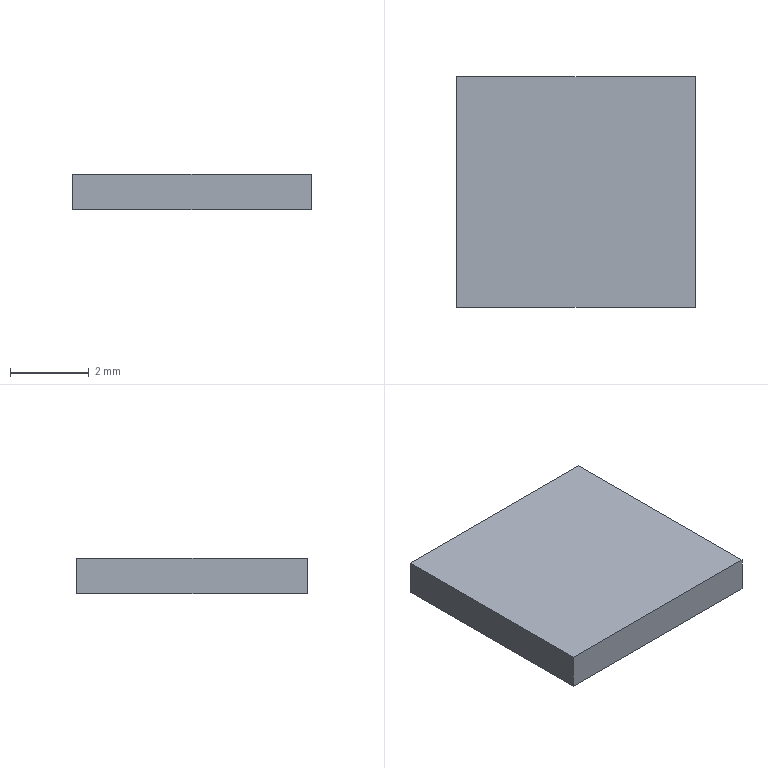Part | Creo | 1 solid | 6 faces | box 6.05 x 5.85 x 0.9 mm | volume 31.853 mm3 | plane 6
STEP:
#1=CARTESIAN_POINT('',(0.,0.,0.));
#2=DIRECTION('',(0.,0.,1.));
#3=DIRECTION('',(1.,0.,0.));
#4=AXIS2_PLACEMENT_3D('',#1,#2,#3);
#5=CARTESIAN_POINT('',(-3.125,-3.025,0.));
#6=VERTEX_POINT('',#5);
#7=CARTESIAN_POINT('',(2.925,-3.025,0.));
#8=VERTEX_POINT('',#7);
#9=CARTESIAN_POINT('',(-3.125,-3.025,0.));
#10=DIRECTION('',(1.,0.,0.));
#11=VECTOR('',#10,6.05);
#12=LINE('',#9,#11);
#13=EDGE_CURVE('',#6,#8,#12,.T.);
#14=ORIENTED_EDGE('',*,*,#13,.T.);
#15=CARTESIAN_POINT('',(2.925,2.825,0.));
#16=VERTEX_POINT('',#15);
#17=CARTESIAN_POINT('',(2.925,-3.025,0.));
#18=DIRECTION('',(0.,1.,0.));
#19=VECTOR('',#18,5.85);
#20=LINE('',#17,#19);
#21=EDGE_CURVE('',#8,#16,#20,.T.);
#22=ORIENTED_EDGE('',*,*,#21,.T.);
#23=CARTESIAN_POINT('',(-3.125,2.825,0.));
#24=VERTEX_POINT('',#23);
#25=CARTESIAN_POINT('',(2.925,2.825,0.));
#26=DIRECTION('',(-1.,0.,0.));
#27=VECTOR('',#26,6.05);
#28=LINE('',#25,#27);
#29=EDGE_CURVE('',#16,#24,#28,.T.);
#30=ORIENTED_EDGE('',*,*,#29,.T.);
#31=CARTESIAN_POINT('',(-3.125,2.825,0.));
#32=DIRECTION('',(0.,-1.,0.));
#33=VECTOR('',#32,5.85);
#34=LINE('',#31,#33);
#35=EDGE_CURVE('',#24,#6,#34,.T.);
#36=ORIENTED_EDGE('',*,*,#35,.T.);
#37=EDGE_LOOP('',(#14,#22,#30,#36));
#38=FACE_OUTER_BOUND('',#37,.F.);
#39=CARTESIAN_POINT('',(0.,0.,0.));
#40=DIRECTION('',(0.,0.,1.));
#41=DIRECTION('',(1.,0.,0.));
#42=AXIS2_PLACEMENT_3D('',#39,#40,#41);
#43=PLANE('',#42);
#44=ADVANCED_FACE('',(#38),#43,.F.);
#45=ORIENTED_EDGE('',*,*,#13,.F.);
#46=CARTESIAN_POINT('',(-3.125,-3.025,0.9));
#47=VERTEX_POINT('',#46);
#48=CARTESIAN_POINT('',(-3.125,-3.025,0.));
#49=DIRECTION('',(0.,0.,1.));
#50=VECTOR('',#49,0.9);
#51=LINE('',#48,#50);
#52=EDGE_CURVE('',#6,#47,#51,.T.);
#53=ORIENTED_EDGE('',*,*,#52,.T.);
#54=CARTESIAN_POINT('',(2.925,-3.025,0.9));
#55=VERTEX_POINT('',#54);
#56=CARTESIAN_POINT('',(-3.125,-3.025,0.9));
#57=DIRECTION('',(1.,0.,0.));
#58=VECTOR('',#57,6.05);
#59=LINE('',#56,#58);
#60=EDGE_CURVE('',#47,#55,#59,.T.);
#61=ORIENTED_EDGE('',*,*,#60,.T.);
#62=CARTESIAN_POINT('',(2.925,-3.025,0.));
#63=DIRECTION('',(0.,0.,1.));
#64=VECTOR('',#63,0.9);
#65=LINE('',#62,#64);
#66=EDGE_CURVE('',#8,#55,#65,.T.);
#67=ORIENTED_EDGE('',*,*,#66,.F.);
#68=EDGE_LOOP('',(#45,#53,#61,#67));
#69=FACE_OUTER_BOUND('',#68,.F.);
#70=CARTESIAN_POINT('',(-3.125,-3.025,0.));
#71=DIRECTION('',(0.,-1.,0.));
#72=DIRECTION('',(1.,0.,0.));
#73=AXIS2_PLACEMENT_3D('',#70,#71,#72);
#74=PLANE('',#73);
#75=ADVANCED_FACE('',(#69),#74,.T.);
#76=ORIENTED_EDGE('',*,*,#35,.F.);
#77=CARTESIAN_POINT('',(-3.125,2.825,0.9));
#78=VERTEX_POINT('',#77);
#79=CARTESIAN_POINT('',(-3.125,2.825,0.));
#80=DIRECTION('',(0.,0.,1.));
#81=VECTOR('',#80,0.9);
#82=LINE('',#79,#81);
#83=EDGE_CURVE('',#24,#78,#82,.T.);
#84=ORIENTED_EDGE('',*,*,#83,.T.);
#85=CARTESIAN_POINT('',(-3.125,2.825,0.9));
#86=DIRECTION('',(0.,-1.,0.));
#87=VECTOR('',#86,5.85);
#88=LINE('',#85,#87);
#89=EDGE_CURVE('',#78,#47,#88,.T.);
#90=ORIENTED_EDGE('',*,*,#89,.T.);
#91=ORIENTED_EDGE('',*,*,#52,.F.);
#92=EDGE_LOOP('',(#76,#84,#90,#91));
#93=FACE_OUTER_BOUND('',#92,.F.);
#94=CARTESIAN_POINT('',(-3.125,2.825,0.));
#95=DIRECTION('',(-1.,0.,0.));
#96=DIRECTION('',(0.,-1.,0.));
#97=AXIS2_PLACEMENT_3D('',#94,#95,#96);
#98=PLANE('',#97);
#99=ADVANCED_FACE('',(#93),#98,.T.);
#100=ORIENTED_EDGE('',*,*,#29,.F.);
#101=CARTESIAN_POINT('',(2.925,2.825,0.9));
#102=VERTEX_POINT('',#101);
#103=CARTESIAN_POINT('',(2.925,2.825,0.));
#104=DIRECTION('',(0.,0.,1.));
#105=VECTOR('',#104,0.9);
#106=LINE('',#103,#105);
#107=EDGE_CURVE('',#16,#102,#106,.T.);
#108=ORIENTED_EDGE('',*,*,#107,.T.);
#109=CARTESIAN_POINT('',(2.925,2.825,0.9));
#110=DIRECTION('',(-1.,0.,0.));
#111=VECTOR('',#110,6.05);
#112=LINE('',#109,#111);
#113=EDGE_CURVE('',#102,#78,#112,.T.);
#114=ORIENTED_EDGE('',*,*,#113,.T.);
#115=ORIENTED_EDGE('',*,*,#83,.F.);
#116=EDGE_LOOP('',(#100,#108,#114,#115));
#117=FACE_OUTER_BOUND('',#116,.F.);
#118=CARTESIAN_POINT('',(2.925,2.825,0.));
#119=DIRECTION('',(0.,1.,0.));
#120=DIRECTION('',(-1.,0.,0.));
#121=AXIS2_PLACEMENT_3D('',#118,#119,#120);
#122=PLANE('',#121);
#123=ADVANCED_FACE('',(#117),#122,.T.);
#124=ORIENTED_EDGE('',*,*,#21,.F.);
#125=ORIENTED_EDGE('',*,*,#66,.T.);
#126=CARTESIAN_POINT('',(2.925,-3.025,0.9));
#127=DIRECTION('',(0.,1.,0.));
#128=VECTOR('',#127,5.85);
#129=LINE('',#126,#128);
#130=EDGE_CURVE('',#55,#102,#129,.T.);
#131=ORIENTED_EDGE('',*,*,#130,.T.);
#132=ORIENTED_EDGE('',*,*,#107,.F.);
#133=EDGE_LOOP('',(#124,#125,#131,#132));
#134=FACE_OUTER_BOUND('',#133,.F.);
#135=CARTESIAN_POINT('',(2.925,-3.025,0.));
#136=DIRECTION('',(1.,0.,0.));
#137=DIRECTION('',(0.,1.,0.));
#138=AXIS2_PLACEMENT_3D('',#135,#136,#137);
#139=PLANE('',#138);
#140=ADVANCED_FACE('',(#134),#139,.T.);
#141=ORIENTED_EDGE('',*,*,#60,.F.);
#142=ORIENTED_EDGE('',*,*,#89,.F.);
#143=ORIENTED_EDGE('',*,*,#113,.F.);
#144=ORIENTED_EDGE('',*,*,#130,.F.);
#145=EDGE_LOOP('',(#141,#142,#143,#144));
#146=FACE_OUTER_BOUND('',#145,.F.);
#147=CARTESIAN_POINT('',(0.,0.,0.9));
#148=DIRECTION('',(0.,0.,1.));
#149=DIRECTION('',(1.,0.,0.));
#150=AXIS2_PLACEMENT_3D('',#147,#148,#149);
#151=PLANE('',#150);
#152=ADVANCED_FACE('',(#146),#151,.T.);
#153=CLOSED_SHELL('',(#44,#75,#99,#123,#140,#152));
#154=MANIFOLD_SOLID_BREP('',#153);
#155=(LENGTH_UNIT()NAMED_UNIT(*)SI_UNIT(.MILLI.,.METRE.));
#156=UNCERTAINTY_MEASURE_WITH_UNIT(LENGTH_MEASURE(0.0008463),#155,'','');
#157=(NAMED_UNIT(*)PLANE_ANGLE_UNIT()SI_UNIT($,.RADIAN.));
#158=PLANE_ANGLE_MEASURE_WITH_UNIT(PLANE_ANGLE_MEASURE(0.01745),#157);
#159=(CONVERSION_BASED_UNIT('DEGREE',#158)NAMED_UNIT(*)PLANE_ANGLE_UNIT());
#160=(NAMED_UNIT(*)SI_UNIT($,.STERADIAN.)SOLID_ANGLE_UNIT());
#161=(GEOMETRIC_REPRESENTATION_CONTEXT(3)GLOBAL_UNCERTAINTY_ASSIGNED_CONTEXT((#156))GLOBAL_UNIT_ASSIGNED_CONTEXT((#155,#159,#160))REPRESENTATION_CONTEXT('',''));
#162=ADVANCED_BREP_SHAPE_REPRESENTATION('',(#4,#154),#161);